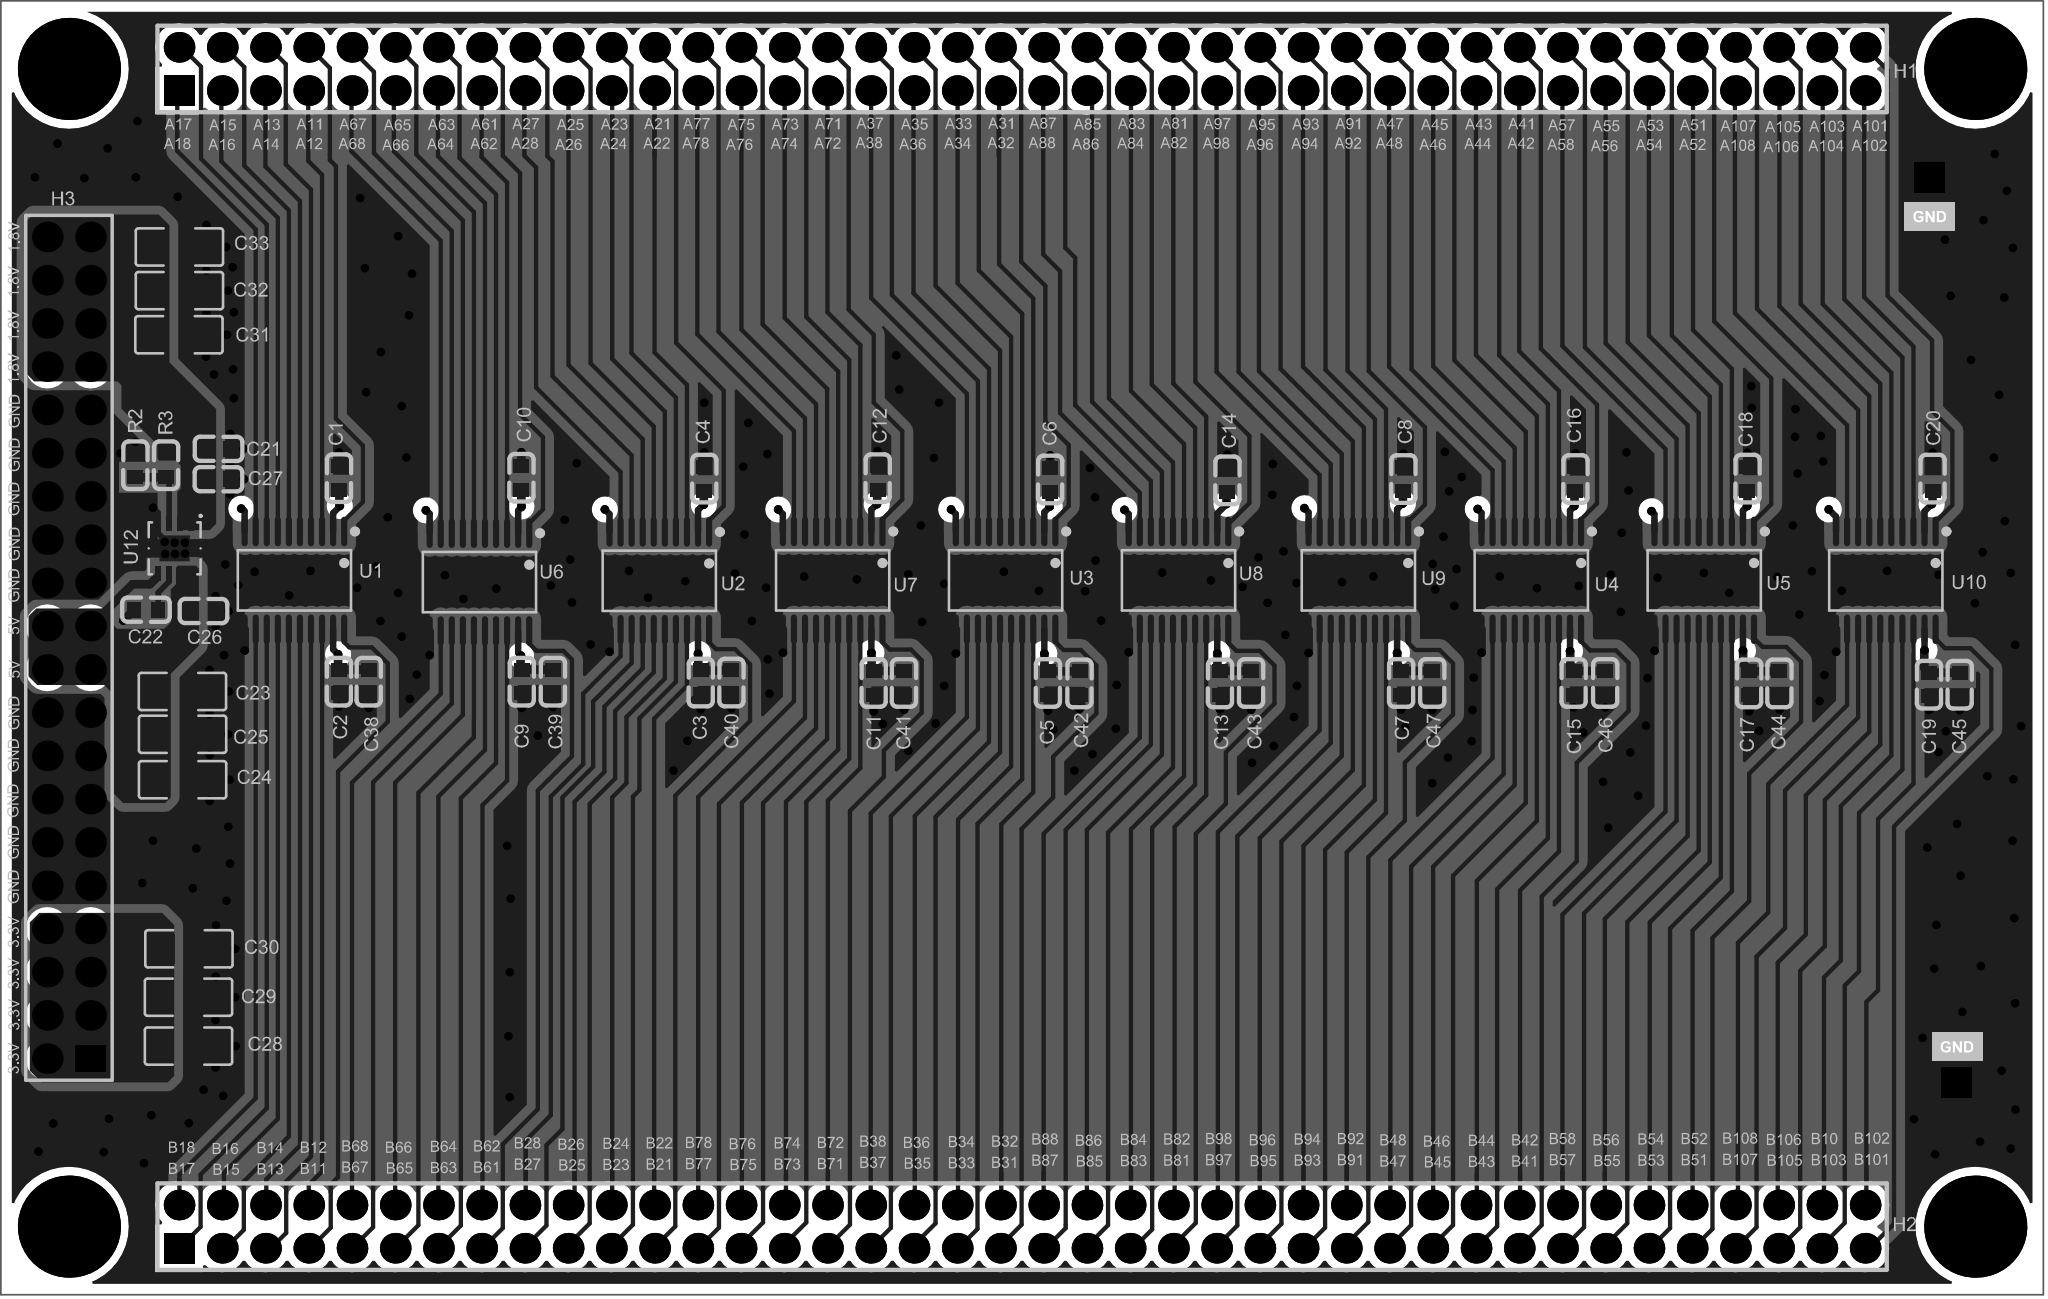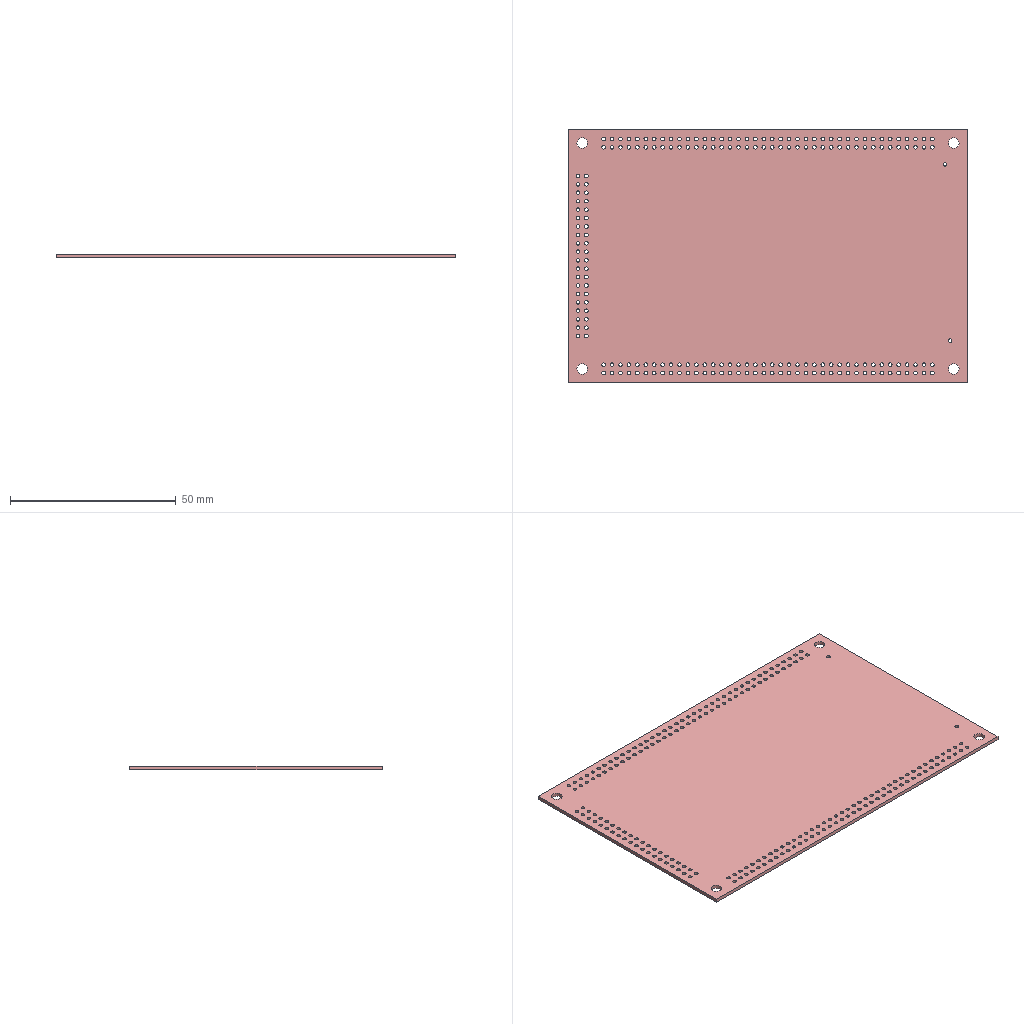Circuit board layout | Altium Designer | box 120 x 76 x 1.1 mm
Layer stack:
# Altium Designer layer stack of  (unit mm; dielectric type: 0 none, 1 core, 2 prepreg, 3 surface material)
index,name,kind,layer,copper_thickness_mm,dielectric_type,dielectric_thickness_mm,dielectric_material,dielectric_constant
0,Top Paste,other,,,,,,
1,Top Overlay,other,,,,,,
2,Top Solder,dielectric,,,3,0.0102,Solder Resist,3.5
3,Top Layer,copper,Top Layer,0.0356,,,,
4,Dielectric1,dielectric,,,1,0.32,FR-4,4.8
5,GND,copper,GND,0.0356,,,,
6,Dielectric5,dielectric,,,2,0.32,FR-4,4.8
7,POWER,copper,POWER,0.0356,,,,
8,Dielectric6,dielectric,,,1,0.32,FR-4,4.8
9,Bottom Layer,copper,Bottom Layer,0.0356,,,,
10,Bottom Solder,dielectric,,,3,0.0102,Solder Resist,3.5
11,Bottom Overlay,other,,,,,,
12,Bottom Paste,other,,,,,,
# drill layer pairs: low layer,high layer
drill_pair,Top Layer,Bottom Layer
Part placement:
Designator,Comment,Layer,Footprint,Center-X(mm),Center-Y(mm),Rotation
C47,4.7u/6.3v,TopLayer,C0603,84.099,35.941,90
C46,4.7u/6.3v,TopLayer,C0603,94.259,35.941,90
C45,4.7u/6.3v,TopLayer,C0603,115.087,35.839,90
C44,4.7u/6.3v,TopLayer,C0603,104.496,35.916,90
C43,4.7u/6.3v,TopLayer,C0603,73.457,35.941,90
C42,4.7u/6.3v,TopLayer,C0603,63.373,35.916,90
C41,4.7u/6.3v,TopLayer,C0603,53.061,35.941,90
C40,4.7u/6.3v,TopLayer,C0603,42.926,35.966,90
C39,4.7u/6.3v,TopLayer,C0603,32.436,36.017,90
C38,4.7u/6.3v,TopLayer,C0603,21.615,36.017,90
C27,4.7u/6.3v,TopLayer,C0603,12.776,47.904,180
C26,1uF/50v,TopLayer,C0603,11.913,40.157,360
C1,0.1u/50V,TopLayer,C0603,19.863,47.955,270
C2,0.1u/50V,TopLayer,C0603,19.863,36.017,90
C3,0.1u/50V,TopLayer,C0603,41.123,35.966,90
C4,0.1u/50V,TopLayer,C0603,41.326,47.93,270
C5,0.1u/50V,TopLayer,C0603,61.519,35.941,90
C6,0.1u/50V,TopLayer,C0603,61.646,47.879,270
C7,0.1u/50V,TopLayer,C0603,82.271,35.941,90
C8,0.1u/50V,TopLayer,C0603,82.398,47.904,270
C9,0.1u/50V,TopLayer,C0603,30.607,36.017,90
C10,0.1u/50V,TopLayer,C0603,30.582,47.981,270
C11,0.1u/50V,TopLayer,C0603,51.283,35.941,90
C12,0.1u/50V,TopLayer,C0603,51.511,47.955,270
C13,0.1u/50V,TopLayer,C0603,71.628,35.916,90
C14,0.1u/50V,TopLayer,C0603,72.06,47.828,270
C15,0.1u/50V,TopLayer,C0603,92.405,35.941,90
C16,0.1u/50V,TopLayer,C0603,92.507,47.904,270
C17,0.1u/50V,TopLayer,C0603,102.718,35.916,90
C18,0.1u/50V,TopLayer,C0603,102.616,47.93,270
C19,0.1u/50V,TopLayer,C0603,113.284,35.839,90
C20,0.1u/50V,TopLayer,C0603,113.487,47.93,270
C21,4.7u/6.3v,TopLayer,C0603,12.783,49.688,180
C22,10nF/50v,TopLayer,C0603,8.534,40.234,360
C23,47uF/10V,TopLayer,C1206,10.668,35.433,180
H1,2.54-2*40,TopLayer,HDR-TH_80P-P2.54-V-M-R2-C40-S2.54,60,72,0
H2,2.54-2*40,TopLayer,HDR-TH_80P-P2.54-V-M-R2-C40-S2.54,60,4,0
H3,B-2100S40P-B110,TopLayer,HDR-TH_40P-P2.54-V-M-R2-C20-S2.54,4,38,90
R2,10k 1%,TopLayer,R0603,7.899,48.717,270
R3,12.5k 1%,TopLayer,R0603,9.703,48.717,270
U1,TXS0108EQPWRQ1,TopLayer,TSSOP-20_L6.5-W4.4-P0.65-LS6.4-BL,17.247,41.961,180
U2,TXS0108EQPWRQ1,TopLayer,TSSOP-20_L6.5-W4.4-P0.65-LS6.4-BL,38.684,41.935,180
U3,TXS0108EQPWRQ1,TopLayer,TSSOP-20_L6.5-W4.4-P0.65-LS6.4-BL,59.03,41.961,180
U4,TXS0108EQPWRQ1,TopLayer,TSSOP-20_L6.5-W4.4-P0.65-LS6.4-BL,89.916,41.961,180
U5,TXS0108EQPWRQ1,TopLayer,TSSOP-20_L6.5-W4.4-P0.65-LS6.4-BL,100.076,41.961,180
U6,TXS0108EQPWRQ1,TopLayer,TSSOP-20_L6.5-W4.4-P0.65-LS6.4-BL,28.118,41.859,180
U7,TXS0108EQPWRQ1,TopLayer,TSSOP-20_L6.5-W4.4-P0.65-LS6.4-BL,48.87,41.961,180
U8,TXS0108EQPWRQ1,TopLayer,TSSOP-20_L6.5-W4.4-P0.65-LS6.4-BL,69.19,41.961,180
U9,TXS0108EQPWRQ1,TopLayer,TSSOP-20_L6.5-W4.4-P0.65-LS6.4-BL,79.756,41.961,180
U10,TXS0108EQPWRQ1,TopLayer,TSSOP-20_L6.5-W4.4-P0.65-LS6.4-BL,110.744,41.961,180
U12,TPS7A8001DRBR,TopLayer,VSON-8_L3.0-W3.0-P0.65-TL-EP,10.211,43.84,270
C24,47uF/10V,TopLayer,C1206,10.676,30.251,180
C25,47uF/10V,TopLayer,C1206,10.676,32.918,180
C28,47uF/10V,TopLayer,C1206,11.024,14.605,180
C29,47uF/10V,TopLayer,C1206,11.024,17.475,180
C30,47uF/10V,TopLayer,C1206,11.049,20.32,180
C31,47uF/10V,TopLayer,C1206,10.462,56.388,180
C32,47uF/10V,TopLayer,C1206,10.49,58.979,180
C33,47uF/10V,TopLayer,C1206,10.49,61.544,180
Pad and via stacks:
# Altium Designer via and pad stacks of  (unit mm). Each distinct definition once, with the count of objects using it.
# via: kind,start_layer,end_layer,hole_mm,diameter_mm,mode(0 simple;1 top-mid-bottom;2 full stack),diameter_per_layer,count,example_net
# pad: kind,layer,hole_mm,hole_type(0 round;1 square;2 slot),plating,top_size,top_shape(1 round;2 rect;3 octagon;9 rounded rect),mid_size,bottom_size,mode,footprint,size_per_layer,count,example
pad,Top Layer,0,0,plated,0.8x0.9,2,0.8x0.9,0.8x0.9,0,C0603,,68,C26.2
pad,Top Layer,0,0,plated,0.34x0.8499,2,0.34x0.8499,0.34x0.8499,0,VSON-8_L3.0-W3.0-P0.65-TL-EP,,8,U12.1
pad,Top Layer,0,0,plated,1.485x1.728,2,1.485x1.728,1.485x1.728,0,C1206,,18,C23.2
pad,Top Layer,0,0,plated,0.364x1.742,1,0.364x1.742,0.364x1.742,0,TSSOP-20_L6.5-W4.4-P0.65-LS6.4-BL,,200,U1.1
pad,Top Layer,0,0,plated,0.8x0.9,2,0.8x0.9,0.8x0.9,0,R0603,,4,R2.2
pad,Multi-Layer,1.1,0,plated,1.8x1.8,2,1.8x1.8,1.8x1.8,0,,,2,1
pad,Multi-Layer,1.1,0,plated,1.8x1.8,2,1.8x1.8,1.8x1.8,0,HDR-TH_80P-P2.54-V-M-R2-C40-S2.54,,2,H1.1
pad,Multi-Layer,1.1,0,plated,1.8x1.8,1,1.8x1.8,1.8x1.8,0,HDR-TH_80P-P2.54-V-M-R2-C40-S2.54,,158,H1.2
pad,Multi-Layer,1.1,0,plated,1.575x1.8,2,1.524x1.524,1.524x1.524,1,HDR-TH_40P-P2.54-V-M-R2-C20-S2.54,,1,H3.1
pad,Multi-Layer,1.1,0,plated,1.8x1.8,1,1.524x1.524,1.524x1.524,1,HDR-TH_40P-P2.54-V-M-R2-C20-S2.54,,39,H3.2
pad,Multi-Layer,3.2,0,plated,6x6,1,6x6,6x6,0,,,4,0
via,Top Layer,Bottom Layer,0.3048,0.508,0,,319,GND
Copper pours:
name,layer,net,type(0 solid;1 hatched;2 none)
Bottom Layer-No Net,Top Layer,GND,0
Bottom Layer-No Net,Top Layer,1.8V,0
Bottom Layer-No Net,Top Layer,+5V,0
Bottom Layer-No Net,Top Layer,3.3V,0
Bottom Layer-No Net,Bottom Layer,GND,0
Design rules, without the lines most boards share:
# Altium Designer design rules of  (exported by Altium Designer, unit mm)
# columns: name | kind | enabled | priority | scope1 | scope2 | descriptor | typed fields (field=value)
Clearance_1 | 0 | enabled | 1 | inpolygon | All | Clearance Constraint (Gap=6mil) (inpolygon),(All) | gap=0.1524
Clearance | 0 | enabled | 2 | All | All | Clearance Constraint (Gap=6mil) (All),(All) | gap=0.1524
PlaneConnect | 6 | enabled | 1 | All | All | Power Plane Connect Rule(Direct Connect )(Expansion=20mil) (Conductor Width=10mil) (Air Gap=10mil) (Entries=4) (All) | relief_conductor_width=0.254 relief_entries=4 relief_expansion=0.508
PlaneClearance | 12 | enabled | 1 | All | All | Power Plane Clearance (Clearance =6mil) (All) | clearance=0.1524
PolygonConnect | 20 | enabled | 1 | All | All | Polygon Connect Rule(Direct Connect )(Conductor Width=10mil) (Relief Angle=90 Angle) (Entries=4) (Air Gap Width=10mil) (All),(All) | connect_style(0=relief,1=direct,2=none)=1 relief_conductor_width=0.254 relief_entries=4
Width | 2 | enabled | 1 | All | All | Width Constraint (Min=8mil) (Max=20mil) (Preferred=8mil) (All) |
RoutingVias | 11 | enabled | 1 | All | All | Routing Via (MinHoleWidth=12mil) (MaxHoleWidth=12mil) (PreferredHoleWidth=12mil) (MinWidth=20mil) (MaxWidth=20mil) (PreferedWidth=20mil) (All) | via_min_hole=0.3048 via_max_hole=0.3048 via_preferred_diameter=0.508 via_preferred_hole=0.3048
SolderMaskExpansion | 13 | enabled | 1 | All | All | Solder Mask Expansion (Expansion =4mil) (All) | expansion=0.1016
HoleSize | 42 | enabled | 1 | All | All | Hole Size Constraint (Min=1mil) (Max=500mil) (All) |
DiffPairsRouting | 51 | enabled | 1 | All | All | Differential Pairs Uncoupled Length using the Gap Constraints (Min=10mil) (Max=10mil) (Prefered=10mil)  and Width Constraints (Min=15mil) (Max=15mil) (Prefered=15mil) (All) |
HoleToHoleClearance | 52 | enabled | 1 | All | All | Hole To Hole Clearance (Gap=0mil) (All),(All) | gap=0
MinimumSolderMaskSliver | 53 | enabled | 1 | All | All | Minimum Solder Mask Sliver (Gap=0mil) (All),(All) |
SilkscreenOverComponentPads | 54 | enabled | 1 | IsPad | All | Silk To Solder Mask (Clearance=0mil) (IsPad),(All) |
SilkToSilkClearance | 55 | enabled | 1 | All | All | Silk to Silk (Clearance=0mil) (All),(All) |
Classes set for this board:
# Altium Designer classes of  (member kind: 0 net, 1 component, 2 from-to, 3 pad, 4 layer, 5 differential pair, 6 design channel, 7 polygon, 8 structure, 9 xSignal)
# columns: class name | member kind | superclass | members
Sheet_1_2023-12-28 | 1 | no | C1; C2; C3; C4; C5; C6; C7; C8; C9; C10; C11; C12; C13; C14; C15; C16; C17; C18; C19; C20; C21; C22; C23; H1; H2; H3; R2; R3; U1; U2; U3; U4; U5; U6; U7; U8; U9; U10; U12; C26; C27; C38; C39; C40; C41; C42; C43; C44; C45; C46; C47; C24; C25; C28; C29; C30; C31; C32; C33;